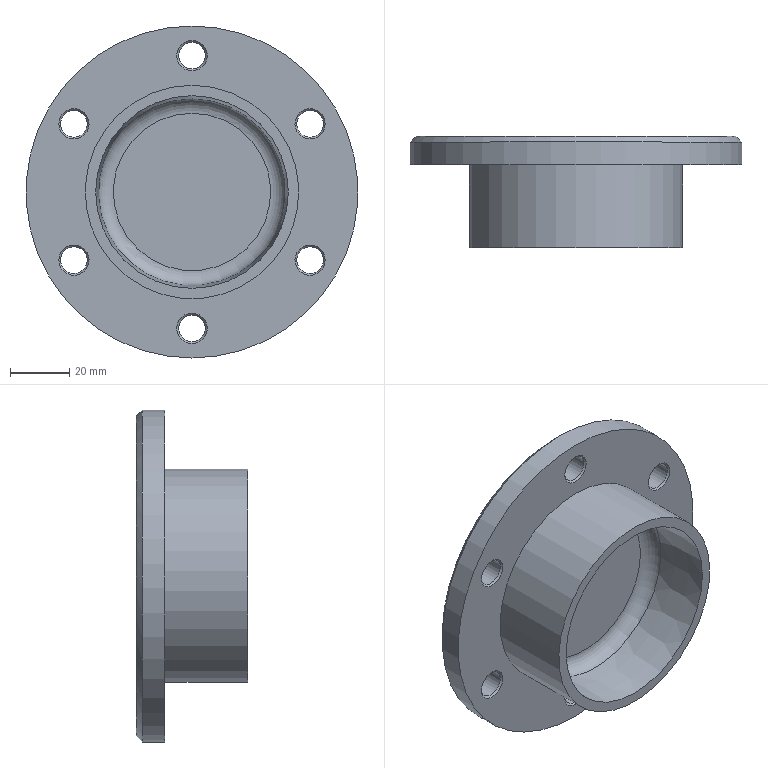Part | NX | 1 solid | 29 faces | box 112 x 37.6 x 112 mm | volume 122481 mm3 | cone 14 | cylinder 8 | plane 5 | torus 2 | commonest cylinder face diameters 9 x6 72 x1 112 x1
STEP:
#1=CARTESIAN_POINT('',(35.94,18.7,-20.75));
#2=VERTEX_POINT('',#1);
#3=CARTESIAN_POINT('',(39.837,18.7,-23.));
#4=DIRECTION('',(0.,1.,0.));
#5=DIRECTION('',(-0.866,0.,0.5));
#6=AXIS2_PLACEMENT_3D('',#3,#4,#5);
#7=CIRCLE('',#6,4.5);
#8=EDGE_CURVE('',#2,#2,#7,.T.);
#9=ORIENTED_EDGE('',*,*,#8,.F.);
#10=EDGE_LOOP('',(#9));
#11=FACE_BOUND('',#10,.T.);
#12=CARTESIAN_POINT('',(35.42,19.3,-20.45));
#13=VERTEX_POINT('',#12);
#14=CARTESIAN_POINT('',(39.837,19.3,-23.));
#15=DIRECTION('',(0.,-1.,0.));
#16=DIRECTION('',(-0.866,0.,0.5));
#17=AXIS2_PLACEMENT_3D('',#14,#15,#16);
#18=CIRCLE('',#17,5.1);
#19=EDGE_CURVE('',#13,#13,#18,.T.);
#20=ORIENTED_EDGE('',*,*,#19,.F.);
#21=EDGE_LOOP('',(#20));
#22=FACE_BOUND('',#21,.T.);
#23=CARTESIAN_POINT('',(39.837,19.3,-23.));
#24=DIRECTION('',(0.,1.,0.));
#25=DIRECTION('',(0.866,0.,-0.5));
#26=AXIS2_PLACEMENT_3D('',#23,#24,#25);
#27=CONICAL_SURFACE('',#26,5.1,45.);
#28=ADVANCED_FACE('',(#11,#22),#27,.F.);
#29=CARTESIAN_POINT('',(44.254,9.7,-25.55));
#30=VERTEX_POINT('',#29);
#31=CARTESIAN_POINT('',(39.837,9.7,-23.));
#32=DIRECTION('',(0.,1.,0.));
#33=DIRECTION('',(0.866,0.,-0.5));
#34=AXIS2_PLACEMENT_3D('',#31,#32,#33);
#35=CIRCLE('',#34,5.1);
#36=EDGE_CURVE('',#30,#30,#35,.T.);
#37=ORIENTED_EDGE('',*,*,#36,.F.);
#38=EDGE_LOOP('',(#37));
#39=FACE_BOUND('',#38,.T.);
#40=CARTESIAN_POINT('',(43.734,10.3,-25.25));
#41=VERTEX_POINT('',#40);
#42=CARTESIAN_POINT('',(39.837,10.3,-23.));
#43=DIRECTION('',(0.,-1.,0.));
#44=DIRECTION('',(0.866,0.,-0.5));
#45=AXIS2_PLACEMENT_3D('',#42,#43,#44);
#46=CIRCLE('',#45,4.5);
#47=EDGE_CURVE('',#41,#41,#46,.T.);
#48=ORIENTED_EDGE('',*,*,#47,.F.);
#49=EDGE_LOOP('',(#48));
#50=FACE_BOUND('',#49,.T.);
#51=CARTESIAN_POINT('',(39.837,10.3,-23.));
#52=DIRECTION('',(0.,-1.,0.));
#53=DIRECTION('',(-0.866,0.,0.5));
#54=AXIS2_PLACEMENT_3D('',#51,#52,#53);
#55=CONICAL_SURFACE('',#54,4.5,45.);
#56=ADVANCED_FACE('',(#39,#50),#55,.F.);
#57=ORIENTED_EDGE('',*,*,#47,.T.);
#58=EDGE_LOOP('',(#57));
#59=FACE_BOUND('',#58,.T.);
#60=ORIENTED_EDGE('',*,*,#8,.T.);
#61=EDGE_LOOP('',(#60));
#62=FACE_BOUND('',#61,.T.);
#63=CARTESIAN_POINT('',(39.837,19.3,-23.));
#64=DIRECTION('',(0.,-1.,0.));
#65=DIRECTION('',(-0.866,0.,0.5));
#66=AXIS2_PLACEMENT_3D('',#63,#64,#65);
#67=CYLINDRICAL_SURFACE('',#66,4.5);
#68=ADVANCED_FACE('',(#59,#62),#67,.F.);
#69=CARTESIAN_POINT('',(35.94,18.7,20.75));
#70=VERTEX_POINT('',#69);
#71=CARTESIAN_POINT('',(39.837,18.7,23.));
#72=DIRECTION('',(0.,1.,0.));
#73=DIRECTION('',(-0.866,0.,-0.5));
#74=AXIS2_PLACEMENT_3D('',#71,#72,#73);
#75=CIRCLE('',#74,4.5);
#76=EDGE_CURVE('',#70,#70,#75,.T.);
#77=ORIENTED_EDGE('',*,*,#76,.F.);
#78=EDGE_LOOP('',(#77));
#79=FACE_BOUND('',#78,.T.);
#80=CARTESIAN_POINT('',(35.42,19.3,20.45));
#81=VERTEX_POINT('',#80);
#82=CARTESIAN_POINT('',(39.837,19.3,23.));
#83=DIRECTION('',(0.,-1.,0.));
#84=DIRECTION('',(-0.866,0.,-0.5));
#85=AXIS2_PLACEMENT_3D('',#82,#83,#84);
#86=CIRCLE('',#85,5.1);
#87=EDGE_CURVE('',#81,#81,#86,.T.);
#88=ORIENTED_EDGE('',*,*,#87,.F.);
#89=EDGE_LOOP('',(#88));
#90=FACE_BOUND('',#89,.T.);
#91=CARTESIAN_POINT('',(39.837,19.3,23.));
#92=DIRECTION('',(0.,1.,0.));
#93=DIRECTION('',(0.866,0.,0.5));
#94=AXIS2_PLACEMENT_3D('',#91,#92,#93);
#95=CONICAL_SURFACE('',#94,5.1,45.);
#96=ADVANCED_FACE('',(#79,#90),#95,.F.);
#97=CARTESIAN_POINT('',(44.254,9.7,25.55));
#98=VERTEX_POINT('',#97);
#99=CARTESIAN_POINT('',(39.837,9.7,23.));
#100=DIRECTION('',(0.,1.,0.));
#101=DIRECTION('',(0.866,0.,0.5));
#102=AXIS2_PLACEMENT_3D('',#99,#100,#101);
#103=CIRCLE('',#102,5.1);
#104=EDGE_CURVE('',#98,#98,#103,.T.);
#105=ORIENTED_EDGE('',*,*,#104,.F.);
#106=EDGE_LOOP('',(#105));
#107=FACE_BOUND('',#106,.T.);
#108=CARTESIAN_POINT('',(43.734,10.3,25.25));
#109=VERTEX_POINT('',#108);
#110=CARTESIAN_POINT('',(39.837,10.3,23.));
#111=DIRECTION('',(0.,-1.,0.));
#112=DIRECTION('',(0.866,0.,0.5));
#113=AXIS2_PLACEMENT_3D('',#110,#111,#112);
#114=CIRCLE('',#113,4.5);
#115=EDGE_CURVE('',#109,#109,#114,.T.);
#116=ORIENTED_EDGE('',*,*,#115,.F.);
#117=EDGE_LOOP('',(#116));
#118=FACE_BOUND('',#117,.T.);
#119=CARTESIAN_POINT('',(39.837,10.3,23.));
#120=DIRECTION('',(0.,-1.,0.));
#121=DIRECTION('',(-0.866,0.,-0.5));
#122=AXIS2_PLACEMENT_3D('',#119,#120,#121);
#123=CONICAL_SURFACE('',#122,4.5,45.);
#124=ADVANCED_FACE('',(#107,#118),#123,.F.);
#125=ORIENTED_EDGE('',*,*,#115,.T.);
#126=EDGE_LOOP('',(#125));
#127=FACE_BOUND('',#126,.T.);
#128=ORIENTED_EDGE('',*,*,#76,.T.);
#129=EDGE_LOOP('',(#128));
#130=FACE_BOUND('',#129,.T.);
#131=CARTESIAN_POINT('',(39.837,19.3,23.));
#132=DIRECTION('',(0.,-1.,0.));
#133=DIRECTION('',(-0.866,0.,-0.5));
#134=AXIS2_PLACEMENT_3D('',#131,#132,#133);
#135=CYLINDRICAL_SURFACE('',#134,4.5);
#136=ADVANCED_FACE('',(#127,#130),#135,.F.);
#137=CARTESIAN_POINT('',(0.,18.7,41.5));
#138=VERTEX_POINT('',#137);
#139=CARTESIAN_POINT('',(0.,18.7,46.));
#140=DIRECTION('',(0.,1.,0.));
#141=DIRECTION('',(0.,0.,-1.));
#142=AXIS2_PLACEMENT_3D('',#139,#140,#141);
#143=CIRCLE('',#142,4.5);
#144=EDGE_CURVE('',#138,#138,#143,.T.);
#145=ORIENTED_EDGE('',*,*,#144,.F.);
#146=EDGE_LOOP('',(#145));
#147=FACE_BOUND('',#146,.T.);
#148=CARTESIAN_POINT('',(0.,19.3,40.9));
#149=VERTEX_POINT('',#148);
#150=CARTESIAN_POINT('',(0.,19.3,46.));
#151=DIRECTION('',(0.,-1.,0.));
#152=DIRECTION('',(0.,0.,-1.));
#153=AXIS2_PLACEMENT_3D('',#150,#151,#152);
#154=CIRCLE('',#153,5.1);
#155=EDGE_CURVE('',#149,#149,#154,.T.);
#156=ORIENTED_EDGE('',*,*,#155,.F.);
#157=EDGE_LOOP('',(#156));
#158=FACE_BOUND('',#157,.T.);
#159=CARTESIAN_POINT('',(0.,19.3,46.));
#160=DIRECTION('',(0.,1.,0.));
#161=DIRECTION('',(0.,0.,1.));
#162=AXIS2_PLACEMENT_3D('',#159,#160,#161);
#163=CONICAL_SURFACE('',#162,5.1,45.);
#164=ADVANCED_FACE('',(#147,#158),#163,.F.);
#165=CARTESIAN_POINT('',(0.,9.7,51.1));
#166=VERTEX_POINT('',#165);
#167=CARTESIAN_POINT('',(0.,9.7,46.));
#168=DIRECTION('',(0.,1.,0.));
#169=DIRECTION('',(0.,0.,1.));
#170=AXIS2_PLACEMENT_3D('',#167,#168,#169);
#171=CIRCLE('',#170,5.1);
#172=EDGE_CURVE('',#166,#166,#171,.T.);
#173=ORIENTED_EDGE('',*,*,#172,.F.);
#174=EDGE_LOOP('',(#173));
#175=FACE_BOUND('',#174,.T.);
#176=CARTESIAN_POINT('',(0.,10.3,50.5));
#177=VERTEX_POINT('',#176);
#178=CARTESIAN_POINT('',(0.,10.3,46.));
#179=DIRECTION('',(0.,-1.,0.));
#180=DIRECTION('',(0.,0.,1.));
#181=AXIS2_PLACEMENT_3D('',#178,#179,#180);
#182=CIRCLE('',#181,4.5);
#183=EDGE_CURVE('',#177,#177,#182,.T.);
#184=ORIENTED_EDGE('',*,*,#183,.F.);
#185=EDGE_LOOP('',(#184));
#186=FACE_BOUND('',#185,.T.);
#187=CARTESIAN_POINT('',(0.,10.3,46.));
#188=DIRECTION('',(0.,-1.,0.));
#189=DIRECTION('',(0.,0.,-1.));
#190=AXIS2_PLACEMENT_3D('',#187,#188,#189);
#191=CONICAL_SURFACE('',#190,4.5,45.);
#192=ADVANCED_FACE('',(#175,#186),#191,.F.);
#193=ORIENTED_EDGE('',*,*,#183,.T.);
#194=EDGE_LOOP('',(#193));
#195=FACE_BOUND('',#194,.T.);
#196=ORIENTED_EDGE('',*,*,#144,.T.);
#197=EDGE_LOOP('',(#196));
#198=FACE_BOUND('',#197,.T.);
#199=CARTESIAN_POINT('',(0.,19.3,46.));
#200=DIRECTION('',(0.,-1.,0.));
#201=DIRECTION('',(0.,0.,-1.));
#202=AXIS2_PLACEMENT_3D('',#199,#200,#201);
#203=CYLINDRICAL_SURFACE('',#202,4.5);
#204=ADVANCED_FACE('',(#195,#198),#203,.F.);
#205=CARTESIAN_POINT('',(-35.94,18.7,20.75));
#206=VERTEX_POINT('',#205);
#207=CARTESIAN_POINT('',(-39.837,18.7,23.));
#208=DIRECTION('',(0.,1.,0.));
#209=DIRECTION('',(0.866,0.,-0.5));
#210=AXIS2_PLACEMENT_3D('',#207,#208,#209);
#211=CIRCLE('',#210,4.5);
#212=EDGE_CURVE('',#206,#206,#211,.T.);
#213=ORIENTED_EDGE('',*,*,#212,.F.);
#214=EDGE_LOOP('',(#213));
#215=FACE_BOUND('',#214,.T.);
#216=CARTESIAN_POINT('',(-35.42,19.3,20.45));
#217=VERTEX_POINT('',#216);
#218=CARTESIAN_POINT('',(-39.837,19.3,23.));
#219=DIRECTION('',(0.,-1.,0.));
#220=DIRECTION('',(0.866,0.,-0.5));
#221=AXIS2_PLACEMENT_3D('',#218,#219,#220);
#222=CIRCLE('',#221,5.1);
#223=EDGE_CURVE('',#217,#217,#222,.T.);
#224=ORIENTED_EDGE('',*,*,#223,.F.);
#225=EDGE_LOOP('',(#224));
#226=FACE_BOUND('',#225,.T.);
#227=CARTESIAN_POINT('',(-39.837,19.3,23.));
#228=DIRECTION('',(0.,1.,0.));
#229=DIRECTION('',(-0.866,0.,0.5));
#230=AXIS2_PLACEMENT_3D('',#227,#228,#229);
#231=CONICAL_SURFACE('',#230,5.1,45.);
#232=ADVANCED_FACE('',(#215,#226),#231,.F.);
#233=CARTESIAN_POINT('',(-44.254,9.7,25.55));
#234=VERTEX_POINT('',#233);
#235=CARTESIAN_POINT('',(-39.837,9.7,23.));
#236=DIRECTION('',(0.,1.,0.));
#237=DIRECTION('',(-0.866,0.,0.5));
#238=AXIS2_PLACEMENT_3D('',#235,#236,#237);
#239=CIRCLE('',#238,5.1);
#240=EDGE_CURVE('',#234,#234,#239,.T.);
#241=ORIENTED_EDGE('',*,*,#240,.F.);
#242=EDGE_LOOP('',(#241));
#243=FACE_BOUND('',#242,.T.);
#244=CARTESIAN_POINT('',(-43.734,10.3,25.25));
#245=VERTEX_POINT('',#244);
#246=CARTESIAN_POINT('',(-39.837,10.3,23.));
#247=DIRECTION('',(0.,-1.,0.));
#248=DIRECTION('',(-0.866,0.,0.5));
#249=AXIS2_PLACEMENT_3D('',#246,#247,#248);
#250=CIRCLE('',#249,4.5);
#251=EDGE_CURVE('',#245,#245,#250,.T.);
#252=ORIENTED_EDGE('',*,*,#251,.F.);
#253=EDGE_LOOP('',(#252));
#254=FACE_BOUND('',#253,.T.);
#255=CARTESIAN_POINT('',(-39.837,10.3,23.));
#256=DIRECTION('',(0.,-1.,0.));
#257=DIRECTION('',(0.866,0.,-0.5));
#258=AXIS2_PLACEMENT_3D('',#255,#256,#257);
#259=CONICAL_SURFACE('',#258,4.5,45.);
#260=ADVANCED_FACE('',(#243,#254),#259,.F.);
#261=ORIENTED_EDGE('',*,*,#251,.T.);
#262=EDGE_LOOP('',(#261));
#263=FACE_BOUND('',#262,.T.);
#264=ORIENTED_EDGE('',*,*,#212,.T.);
#265=EDGE_LOOP('',(#264));
#266=FACE_BOUND('',#265,.T.);
#267=CARTESIAN_POINT('',(-39.837,19.3,23.));
#268=DIRECTION('',(0.,-1.,0.));
#269=DIRECTION('',(0.866,0.,-0.5));
#270=AXIS2_PLACEMENT_3D('',#267,#268,#269);
#271=CYLINDRICAL_SURFACE('',#270,4.5);
#272=ADVANCED_FACE('',(#263,#266),#271,.F.);
#273=CARTESIAN_POINT('',(-35.94,18.7,-20.75));
#274=VERTEX_POINT('',#273);
#275=CARTESIAN_POINT('',(-39.837,18.7,-23.));
#276=DIRECTION('',(0.,1.,0.));
#277=DIRECTION('',(0.866,0.,0.5));
#278=AXIS2_PLACEMENT_3D('',#275,#276,#277);
#279=CIRCLE('',#278,4.5);
#280=EDGE_CURVE('',#274,#274,#279,.T.);
#281=ORIENTED_EDGE('',*,*,#280,.F.);
#282=EDGE_LOOP('',(#281));
#283=FACE_BOUND('',#282,.T.);
#284=CARTESIAN_POINT('',(-35.42,19.3,-20.45));
#285=VERTEX_POINT('',#284);
#286=CARTESIAN_POINT('',(-39.837,19.3,-23.));
#287=DIRECTION('',(0.,-1.,0.));
#288=DIRECTION('',(0.866,0.,0.5));
#289=AXIS2_PLACEMENT_3D('',#286,#287,#288);
#290=CIRCLE('',#289,5.1);
#291=EDGE_CURVE('',#285,#285,#290,.T.);
#292=ORIENTED_EDGE('',*,*,#291,.F.);
#293=EDGE_LOOP('',(#292));
#294=FACE_BOUND('',#293,.T.);
#295=CARTESIAN_POINT('',(-39.837,19.3,-23.));
#296=DIRECTION('',(0.,1.,0.));
#297=DIRECTION('',(-0.866,0.,-0.5));
#298=AXIS2_PLACEMENT_3D('',#295,#296,#297);
#299=CONICAL_SURFACE('',#298,5.1,45.);
#300=ADVANCED_FACE('',(#283,#294),#299,.F.);
#301=CARTESIAN_POINT('',(-44.254,9.7,-25.55));
#302=VERTEX_POINT('',#301);
#303=CARTESIAN_POINT('',(-39.837,9.7,-23.));
#304=DIRECTION('',(0.,1.,0.));
#305=DIRECTION('',(-0.866,0.,-0.5));
#306=AXIS2_PLACEMENT_3D('',#303,#304,#305);
#307=CIRCLE('',#306,5.1);
#308=EDGE_CURVE('',#302,#302,#307,.T.);
#309=ORIENTED_EDGE('',*,*,#308,.F.);
#310=EDGE_LOOP('',(#309));
#311=FACE_BOUND('',#310,.T.);
#312=CARTESIAN_POINT('',(-43.734,10.3,-25.25));
#313=VERTEX_POINT('',#312);
#314=CARTESIAN_POINT('',(-39.837,10.3,-23.));
#315=DIRECTION('',(0.,-1.,0.));
#316=DIRECTION('',(-0.866,0.,-0.5));
#317=AXIS2_PLACEMENT_3D('',#314,#315,#316);
#318=CIRCLE('',#317,4.5);
#319=EDGE_CURVE('',#313,#313,#318,.T.);
#320=ORIENTED_EDGE('',*,*,#319,.F.);
#321=EDGE_LOOP('',(#320));
#322=FACE_BOUND('',#321,.T.);
#323=CARTESIAN_POINT('',(-39.837,10.3,-23.));
#324=DIRECTION('',(0.,-1.,0.));
#325=DIRECTION('',(0.866,0.,0.5));
#326=AXIS2_PLACEMENT_3D('',#323,#324,#325);
#327=CONICAL_SURFACE('',#326,4.5,45.);
#328=ADVANCED_FACE('',(#311,#322),#327,.F.);
#329=ORIENTED_EDGE('',*,*,#319,.T.);
#330=EDGE_LOOP('',(#329));
#331=FACE_BOUND('',#330,.T.);
#332=ORIENTED_EDGE('',*,*,#280,.T.);
#333=EDGE_LOOP('',(#332));
#334=FACE_BOUND('',#333,.T.);
#335=CARTESIAN_POINT('',(-39.837,19.3,-23.));
#336=DIRECTION('',(0.,-1.,0.));
#337=DIRECTION('',(0.866,0.,0.5));
#338=AXIS2_PLACEMENT_3D('',#335,#336,#337);
#339=CYLINDRICAL_SURFACE('',#338,4.5);
#340=ADVANCED_FACE('',(#331,#334),#339,.F.);
#341=CARTESIAN_POINT('',(0.,5.3,26.564));
#342=VERTEX_POINT('',#341);
#343=CARTESIAN_POINT('',(0.,5.3,0.));
#344=DIRECTION('',(0.,1.,0.));
#345=DIRECTION('',(0.,0.,1.));
#346=AXIS2_PLACEMENT_3D('',#343,#344,#345);
#347=CIRCLE('',#346,26.564);
#348=EDGE_CURVE('',#342,#342,#347,.T.);
#349=ORIENTED_EDGE('',*,*,#348,.F.);
#350=EDGE_LOOP('',(#349));
#351=FACE_OUTER_BOUND('',#350,.T.);
#352=CARTESIAN_POINT('',(26.564,5.3,0.));
#353=DIRECTION('',(0.,-1.,0.));
#354=DIRECTION('',(0.,0.,1.));
#355=AXIS2_PLACEMENT_3D('',#352,#353,#354);
#356=PLANE('',#355);
#357=ADVANCED_FACE('',(#351),#356,.T.);
#358=ORIENTED_EDGE('',*,*,#348,.T.);
#359=EDGE_LOOP('',(#358));
#360=FACE_BOUND('',#359,.T.);
#361=CARTESIAN_POINT('',(0.,0.5497,31.558));
#362=VERTEX_POINT('',#361);
#363=CARTESIAN_POINT('',(0.,0.5497,0.));
#364=DIRECTION('',(0.,1.,0.));
#365=DIRECTION('',(0.,0.,1.));
#366=AXIS2_PLACEMENT_3D('',#363,#364,#365);
#367=CIRCLE('',#366,31.558);
#368=EDGE_CURVE('',#362,#362,#367,.T.);
#369=ORIENTED_EDGE('',*,*,#368,.F.);
#370=EDGE_LOOP('',(#369));
#371=FACE_BOUND('',#370,.T.);
#372=CARTESIAN_POINT('',(0.,0.3,0.));
#373=DIRECTION('',(0.,1.,0.));
#374=DIRECTION('',(0.,0.,-1.));
#375=AXIS2_PLACEMENT_3D('',#372,#373,#374);
#376=TOROIDAL_SURFACE('',#375,26.564,5.);
#377=ADVANCED_FACE('',(#360,#371),#376,.F.);
#378=ORIENTED_EDGE('',*,*,#368,.T.);
#379=EDGE_LOOP('',(#378));
#380=FACE_BOUND('',#379,.T.);
#381=CARTESIAN_POINT('',(0.,-18.3,32.5));
#382=VERTEX_POINT('',#381);
#383=CARTESIAN_POINT('',(0.,-18.3,0.));
#384=DIRECTION('',(0.,1.,0.));
#385=DIRECTION('',(0.,0.,1.));
#386=AXIS2_PLACEMENT_3D('',#383,#384,#385);
#387=CIRCLE('',#386,32.5);
#388=EDGE_CURVE('',#382,#382,#387,.T.);
#389=ORIENTED_EDGE('',*,*,#388,.F.);
#390=EDGE_LOOP('',(#389));
#391=FACE_BOUND('',#390,.T.);
#392=CARTESIAN_POINT('',(0.,-18.3,0.));
#393=DIRECTION('',(0.,-1.,0.));
#394=DIRECTION('',(0.,0.,1.));
#395=AXIS2_PLACEMENT_3D('',#392,#393,#394);
#396=CONICAL_SURFACE('',#395,32.5,2.862);
#397=ADVANCED_FACE('',(#380,#391),#396,.F.);
#398=ORIENTED_EDGE('',*,*,#388,.T.);
#399=EDGE_LOOP('',(#398));
#400=FACE_BOUND('',#399,.T.);
#401=CARTESIAN_POINT('',(0.,-18.3,36.));
#402=VERTEX_POINT('',#401);
#403=CARTESIAN_POINT('',(0.,-18.3,0.));
#404=DIRECTION('',(0.,1.,0.));
#405=DIRECTION('',(0.,0.,1.));
#406=AXIS2_PLACEMENT_3D('',#403,#404,#405);
#407=CIRCLE('',#406,36.);
#408=EDGE_CURVE('',#402,#402,#407,.T.);
#409=ORIENTED_EDGE('',*,*,#408,.F.);
#410=EDGE_LOOP('',(#409));
#411=FACE_BOUND('',#410,.T.);
#412=CARTESIAN_POINT('',(36.,-18.3,0.));
#413=DIRECTION('',(0.,-1.,0.));
#414=DIRECTION('',(0.,0.,1.));
#415=AXIS2_PLACEMENT_3D('',#412,#413,#414);
#416=PLANE('',#415);
#417=ADVANCED_FACE('',(#400,#411),#416,.T.);
#418=ORIENTED_EDGE('',*,*,#408,.T.);
#419=EDGE_LOOP('',(#418));
#420=FACE_BOUND('',#419,.T.);
#421=CARTESIAN_POINT('',(0.,9.7,36.));
#422=VERTEX_POINT('',#421);
#423=CARTESIAN_POINT('',(0.,9.7,0.));
#424=DIRECTION('',(0.,1.,0.));
#425=DIRECTION('',(0.,0.,1.));
#426=AXIS2_PLACEMENT_3D('',#423,#424,#425);
#427=CIRCLE('',#426,36.);
#428=EDGE_CURVE('',#422,#422,#427,.T.);
#429=ORIENTED_EDGE('',*,*,#428,.F.);
#430=EDGE_LOOP('',(#429));
#431=FACE_BOUND('',#430,.T.);
#432=CARTESIAN_POINT('',(0.,30.,0.));
#433=DIRECTION('',(0.,1.,0.));
#434=DIRECTION('',(0.,0.,-1.));
#435=AXIS2_PLACEMENT_3D('',#432,#433,#434);
#436=CYLINDRICAL_SURFACE('',#435,36.);
#437=ADVANCED_FACE('',(#420,#431),#436,.T.);
#438=ORIENTED_EDGE('',*,*,#36,.T.);
#439=EDGE_LOOP('',(#438));
#440=FACE_BOUND('',#439,.T.);
#441=ORIENTED_EDGE('',*,*,#104,.T.);
#442=EDGE_LOOP('',(#441));
#443=FACE_BOUND('',#442,.T.);
#444=ORIENTED_EDGE('',*,*,#172,.T.);
#445=EDGE_LOOP('',(#444));
#446=FACE_BOUND('',#445,.T.);
#447=ORIENTED_EDGE('',*,*,#240,.T.);
#448=EDGE_LOOP('',(#447));
#449=FACE_BOUND('',#448,.T.);
#450=ORIENTED_EDGE('',*,*,#308,.T.);
#451=EDGE_LOOP('',(#450));
#452=FACE_BOUND('',#451,.T.);
#453=CARTESIAN_POINT('',(0.,9.7,-51.1));
#454=VERTEX_POINT('',#453);
#455=CARTESIAN_POINT('',(0.,9.7,-46.));
#456=DIRECTION('',(0.,1.,0.));
#457=DIRECTION('',(0.,0.,-1.));
#458=AXIS2_PLACEMENT_3D('',#455,#456,#457);
#459=CIRCLE('',#458,5.1);
#460=EDGE_CURVE('',#454,#454,#459,.T.);
#461=ORIENTED_EDGE('',*,*,#460,.T.);
#462=EDGE_LOOP('',(#461));
#463=FACE_BOUND('',#462,.T.);
#464=ORIENTED_EDGE('',*,*,#428,.T.);
#465=EDGE_LOOP('',(#464));
#466=FACE_BOUND('',#465,.T.);
#467=CARTESIAN_POINT('',(0.,9.7,56.));
#468=VERTEX_POINT('',#467);
#469=CARTESIAN_POINT('',(0.,9.7,0.));
#470=DIRECTION('',(0.,1.,0.));
#471=DIRECTION('',(0.,0.,1.));
#472=AXIS2_PLACEMENT_3D('',#469,#470,#471);
#473=CIRCLE('',#472,56.);
#474=EDGE_CURVE('',#468,#468,#473,.T.);
#475=ORIENTED_EDGE('',*,*,#474,.F.);
#476=EDGE_LOOP('',(#475));
#477=FACE_BOUND('',#476,.T.);
#478=CARTESIAN_POINT('',(56.,9.7,0.));
#479=DIRECTION('',(0.,-1.,0.));
#480=DIRECTION('',(0.,0.,1.));
#481=AXIS2_PLACEMENT_3D('',#478,#479,#480);
#482=PLANE('',#481);
#483=ADVANCED_FACE('',(#440,#443,#446,#449,#452,#463,#466,#477),#482,.T.);
#484=ORIENTED_EDGE('',*,*,#474,.T.);
#485=EDGE_LOOP('',(#484));
#486=FACE_BOUND('',#485,.T.);
#487=CARTESIAN_POINT('',(0.,17.3,56.));
#488=VERTEX_POINT('',#487);
#489=CARTESIAN_POINT('',(0.,17.3,0.));
#490=DIRECTION('',(0.,1.,0.));
#491=DIRECTION('',(0.,0.,1.));
#492=AXIS2_PLACEMENT_3D('',#489,#490,#491);
#493=CIRCLE('',#492,56.);
#494=EDGE_CURVE('',#488,#488,#493,.T.);
#495=ORIENTED_EDGE('',*,*,#494,.F.);
#496=EDGE_LOOP('',(#495));
#497=FACE_BOUND('',#496,.T.);
#498=CARTESIAN_POINT('',(0.,30.,0.));
#499=DIRECTION('',(0.,1.,0.));
#500=DIRECTION('',(0.,0.,-1.));
#501=AXIS2_PLACEMENT_3D('',#498,#499,#500);
#502=CYLINDRICAL_SURFACE('',#501,56.);
#503=ADVANCED_FACE('',(#486,#497),#502,.T.);
#504=ORIENTED_EDGE('',*,*,#494,.T.);
#505=EDGE_LOOP('',(#504));
#506=FACE_BOUND('',#505,.T.);
#507=CARTESIAN_POINT('',(0.,19.3,54.));
#508=VERTEX_POINT('',#507);
#509=CARTESIAN_POINT('',(0.,19.3,0.));
#510=DIRECTION('',(0.,1.,0.));
#511=DIRECTION('',(0.,0.,1.));
#512=AXIS2_PLACEMENT_3D('',#509,#510,#511);
#513=CIRCLE('',#512,54.);
#514=EDGE_CURVE('',#508,#508,#513,.T.);
#515=ORIENTED_EDGE('',*,*,#514,.F.);
#516=EDGE_LOOP('',(#515));
#517=FACE_BOUND('',#516,.T.);
#518=CARTESIAN_POINT('',(0.,19.3,0.));
#519=DIRECTION('',(0.,-1.,0.));
#520=DIRECTION('',(0.,0.,1.));
#521=AXIS2_PLACEMENT_3D('',#518,#519,#520);
#522=CONICAL_SURFACE('',#521,54.,45.);
#523=ADVANCED_FACE('',(#506,#517),#522,.T.);
#524=ORIENTED_EDGE('',*,*,#19,.T.);
#525=EDGE_LOOP('',(#524));
#526=FACE_BOUND('',#525,.T.);
#527=ORIENTED_EDGE('',*,*,#87,.T.);
#528=EDGE_LOOP('',(#527));
#529=FACE_BOUND('',#528,.T.);
#530=ORIENTED_EDGE('',*,*,#155,.T.);
#531=EDGE_LOOP('',(#530));
#532=FACE_BOUND('',#531,.T.);
#533=ORIENTED_EDGE('',*,*,#223,.T.);
#534=EDGE_LOOP('',(#533));
#535=FACE_BOUND('',#534,.T.);
#536=ORIENTED_EDGE('',*,*,#291,.T.);
#537=EDGE_LOOP('',(#536));
#538=FACE_BOUND('',#537,.T.);
#539=CARTESIAN_POINT('',(0.,19.3,-40.9));
#540=VERTEX_POINT('',#539);
#541=CARTESIAN_POINT('',(0.,19.3,-46.));
#542=DIRECTION('',(0.,-1.,0.));
#543=DIRECTION('',(0.,0.,1.));
#544=AXIS2_PLACEMENT_3D('',#541,#542,#543);
#545=CIRCLE('',#544,5.1);
#546=EDGE_CURVE('',#540,#540,#545,.T.);
#547=ORIENTED_EDGE('',*,*,#546,.T.);
#548=EDGE_LOOP('',(#547));
#549=FACE_BOUND('',#548,.T.);
#550=ORIENTED_EDGE('',*,*,#514,.T.);
#551=EDGE_LOOP('',(#550));
#552=FACE_BOUND('',#551,.T.);
#553=CARTESIAN_POINT('',(0.,19.3,34.));
#554=VERTEX_POINT('',#553);
#555=CARTESIAN_POINT('',(0.,19.3,0.));
#556=DIRECTION('',(0.,1.,0.));
#557=DIRECTION('',(0.,0.,1.));
#558=AXIS2_PLACEMENT_3D('',#555,#556,#557);
#559=CIRCLE('',#558,34.);
#560=EDGE_CURVE('',#554,#554,#559,.T.);
#561=ORIENTED_EDGE('',*,*,#560,.F.);
#562=EDGE_LOOP('',(#561));
#563=FACE_BOUND('',#562,.T.);
#564=CARTESIAN_POINT('',(34.,19.3,0.));
#565=DIRECTION('',(0.,1.,0.));
#566=DIRECTION('',(0.,0.,-1.));
#567=AXIS2_PLACEMENT_3D('',#564,#565,#566);
#568=PLANE('',#567);
#569=ADVANCED_FACE('',(#526,#529,#532,#535,#538,#549,#552,#563),#568,.T.);
#570=ORIENTED_EDGE('',*,*,#560,.T.);
#571=EDGE_LOOP('',(#570));
#572=FACE_BOUND('',#571,.T.);
#573=CARTESIAN_POINT('',(0.,17.3,32.));
#574=VERTEX_POINT('',#573);
#575=CARTESIAN_POINT('',(0.,17.3,0.));
#576=DIRECTION('',(0.,1.,0.));
#577=DIRECTION('',(0.,0.,1.));
#578=AXIS2_PLACEMENT_3D('',#575,#576,#577);
#579=CIRCLE('',#578,32.);
#580=EDGE_CURVE('',#574,#574,#579,.T.);
#581=ORIENTED_EDGE('',*,*,#580,.F.);
#582=EDGE_LOOP('',(#581));
#583=FACE_BOUND('',#582,.T.);
#584=CARTESIAN_POINT('',(0.,19.3,0.));
#585=DIRECTION('',(0.,1.,0.));
#586=DIRECTION('',(0.,0.,-1.));
#587=AXIS2_PLACEMENT_3D('',#584,#585,#586);
#588=TOROIDAL_SURFACE('',#587,32.,2.);
#589=ADVANCED_FACE('',(#572,#583),#588,.F.);
#590=ORIENTED_EDGE('',*,*,#580,.T.);
#591=EDGE_LOOP('',(#590));
#592=FACE_OUTER_BOUND('',#591,.T.);
#593=CARTESIAN_POINT('',(0.,17.3,0.));
#594=DIRECTION('',(0.,1.,0.));
#595=DIRECTION('',(0.,0.,-1.));
#596=AXIS2_PLACEMENT_3D('',#593,#594,#595);
#597=PLANE('',#596);
#598=ADVANCED_FACE('',(#592),#597,.T.);
#599=CARTESIAN_POINT('',(0.,10.3,-50.5));
#600=VERTEX_POINT('',#599);
#601=CARTESIAN_POINT('',(0.,10.3,-46.));
#602=DIRECTION('',(0.,-1.,0.));
#603=DIRECTION('',(0.,0.,-1.));
#604=AXIS2_PLACEMENT_3D('',#601,#602,#603);
#605=CIRCLE('',#604,4.5);
#606=EDGE_CURVE('',#600,#600,#605,.T.);
#607=ORIENTED_EDGE('',*,*,#606,.T.);
#608=EDGE_LOOP('',(#607));
#609=FACE_BOUND('',#608,.T.);
#610=CARTESIAN_POINT('',(0.,18.7,-41.5));
#611=VERTEX_POINT('',#610);
#612=CARTESIAN_POINT('',(0.,18.7,-46.));
#613=DIRECTION('',(0.,1.,0.));
#614=DIRECTION('',(0.,0.,1.));
#615=AXIS2_PLACEMENT_3D('',#612,#613,#614);
#616=CIRCLE('',#615,4.5);
#617=EDGE_CURVE('',#611,#611,#616,.T.);
#618=ORIENTED_EDGE('',*,*,#617,.T.);
#619=EDGE_LOOP('',(#618));
#620=FACE_BOUND('',#619,.T.);
#621=CARTESIAN_POINT('',(0.,19.3,-46.));
#622=DIRECTION('',(0.,-1.,0.));
#623=DIRECTION('',(0.,0.,1.));
#624=AXIS2_PLACEMENT_3D('',#621,#622,#623);
#625=CYLINDRICAL_SURFACE('',#624,4.5);
#626=ADVANCED_FACE('',(#609,#620),#625,.F.);
#627=ORIENTED_EDGE('',*,*,#617,.F.);
#628=EDGE_LOOP('',(#627));
#629=FACE_BOUND('',#628,.T.);
#630=ORIENTED_EDGE('',*,*,#546,.F.);
#631=EDGE_LOOP('',(#630));
#632=FACE_BOUND('',#631,.T.);
#633=CARTESIAN_POINT('',(0.,19.3,-46.));
#634=DIRECTION('',(0.,1.,0.));
#635=DIRECTION('',(0.,0.,-1.));
#636=AXIS2_PLACEMENT_3D('',#633,#634,#635);
#637=CONICAL_SURFACE('',#636,5.1,45.);
#638=ADVANCED_FACE('',(#629,#632),#637,.F.);
#639=ORIENTED_EDGE('',*,*,#460,.F.);
#640=EDGE_LOOP('',(#639));
#641=FACE_BOUND('',#640,.T.);
#642=ORIENTED_EDGE('',*,*,#606,.F.);
#643=EDGE_LOOP('',(#642));
#644=FACE_BOUND('',#643,.T.);
#645=CARTESIAN_POINT('',(0.,10.3,-46.));
#646=DIRECTION('',(0.,-1.,0.));
#647=DIRECTION('',(0.,0.,1.));
#648=AXIS2_PLACEMENT_3D('',#645,#646,#647);
#649=CONICAL_SURFACE('',#648,4.5,45.);
#650=ADVANCED_FACE('',(#641,#644),#649,.F.);
#651=CLOSED_SHELL('',(#28,#56,#68,#96,#124,#136,#164,#192,#204,#232,#260,#272,#300,#328,#340,#357,#377,#397,#417,#437,#483,#503,#523,#569,#589,#598,#626,#638,#650));
#652=MANIFOLD_SOLID_BREP('',#651);
#653=(LENGTH_UNIT()NAMED_UNIT(*)SI_UNIT(.MILLI.,.METRE.));
#654=UNCERTAINTY_MEASURE_WITH_UNIT(LENGTH_MEASURE(0.00002),#653,'','');
#655=(NAMED_UNIT(*)PLANE_ANGLE_UNIT()SI_UNIT($,.RADIAN.));
#656=PLANE_ANGLE_MEASURE_WITH_UNIT(PLANE_ANGLE_MEASURE(0.01745),#655);
#657=DIMENSIONAL_EXPONENTS(0.,0.,0.,0.,0.,0.,0.);
#658=(CONVERSION_BASED_UNIT('DEGREE',#656)NAMED_UNIT(#657)PLANE_ANGLE_UNIT());
#659=(NAMED_UNIT(*)SI_UNIT($,.STERADIAN.)SOLID_ANGLE_UNIT());
#660=(GEOMETRIC_REPRESENTATION_CONTEXT(3)GLOBAL_UNCERTAINTY_ASSIGNED_CONTEXT((#654))GLOBAL_UNIT_ASSIGNED_CONTEXT((#653,#658,#659))REPRESENTATION_CONTEXT('',''));
#661=ADVANCED_BREP_SHAPE_REPRESENTATION('',(#652),#660);